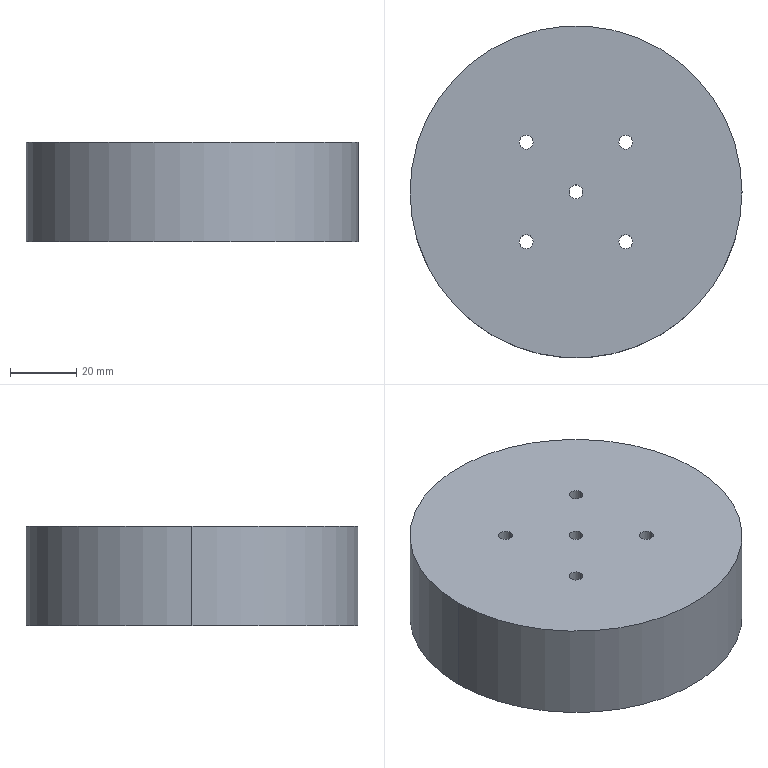Part | SolidWorks | features Extrusion 1, HoleWzd 1 | 1 solid | 14 faces | box 100 x 100 x 30 mm | volume 233541 mm3 | cylinder 12 | plane 2 | commonest cylinder face diameters 4.2 x10 100 x2
STEP:
#1=CARTESIAN_POINT('',(2.1,0.,30.));
#2=VERTEX_POINT('',#1);
#3=CARTESIAN_POINT('',(-2.1,0.,30.));
#4=VERTEX_POINT('',#3);
#5=CARTESIAN_POINT('',(0.,0.,30.));
#6=DIRECTION('',(0.,0.,-1.));
#7=DIRECTION('',(-1.,0.,0.));
#8=AXIS2_PLACEMENT_3D('',#5,#6,#7);
#9=CIRCLE('',#8,2.1);
#10=EDGE_CURVE('',#2,#4,#9,.T.);
#11=ORIENTED_EDGE('',*,*,#10,.F.);
#12=CARTESIAN_POINT('',(2.1,0.,0.));
#13=VERTEX_POINT('',#12);
#14=CARTESIAN_POINT('',(2.1,0.,0.));
#15=DIRECTION('',(0.,0.,-1.));
#16=VECTOR('',#15,1000.);
#17=LINE('',#14,#16);
#18=EDGE_CURVE('',#2,#13,#17,.T.);
#19=ORIENTED_EDGE('',*,*,#18,.T.);
#20=CARTESIAN_POINT('',(-2.1,0.,0.));
#21=VERTEX_POINT('',#20);
#22=CARTESIAN_POINT('',(0.,0.,0.));
#23=DIRECTION('',(0.,0.,-1.));
#24=DIRECTION('',(-1.,0.,0.));
#25=AXIS2_PLACEMENT_3D('',#22,#23,#24);
#26=CIRCLE('',#25,2.1);
#27=EDGE_CURVE('',#13,#21,#26,.T.);
#28=ORIENTED_EDGE('',*,*,#27,.T.);
#29=CARTESIAN_POINT('',(-2.1,0.,0.));
#30=DIRECTION('',(0.,0.,-1.));
#31=VECTOR('',#30,1000.);
#32=LINE('',#29,#31);
#33=EDGE_CURVE('',#4,#21,#32,.T.);
#34=ORIENTED_EDGE('',*,*,#33,.F.);
#35=EDGE_LOOP('',(#11,#19,#28,#34));
#36=FACE_OUTER_BOUND('',#35,.T.);
#37=CARTESIAN_POINT('',(0.,0.,0.));
#38=DIRECTION('',(0.,0.,-1.));
#39=DIRECTION('',(-1.,0.,0.));
#40=AXIS2_PLACEMENT_3D('',#37,#38,#39);
#41=CYLINDRICAL_SURFACE('',#40,2.1);
#42=ADVANCED_FACE('',(#36),#41,.F.);
#43=CARTESIAN_POINT('',(-12.9,-15.,30.));
#44=VERTEX_POINT('',#43);
#45=CARTESIAN_POINT('',(-17.1,-15.,30.));
#46=VERTEX_POINT('',#45);
#47=CARTESIAN_POINT('',(-15.,-15.,30.));
#48=DIRECTION('',(0.,0.,-1.));
#49=DIRECTION('',(-1.,0.,0.));
#50=AXIS2_PLACEMENT_3D('',#47,#48,#49);
#51=CIRCLE('',#50,2.1);
#52=EDGE_CURVE('',#44,#46,#51,.T.);
#53=ORIENTED_EDGE('',*,*,#52,.F.);
#54=CARTESIAN_POINT('',(-12.9,-15.,0.));
#55=VERTEX_POINT('',#54);
#56=CARTESIAN_POINT('',(-12.9,-15.,0.));
#57=DIRECTION('',(0.,0.,-1.));
#58=VECTOR('',#57,1000.);
#59=LINE('',#56,#58);
#60=EDGE_CURVE('',#44,#55,#59,.T.);
#61=ORIENTED_EDGE('',*,*,#60,.T.);
#62=CARTESIAN_POINT('',(-17.1,-15.,0.));
#63=VERTEX_POINT('',#62);
#64=CARTESIAN_POINT('',(-15.,-15.,0.));
#65=DIRECTION('',(0.,0.,-1.));
#66=DIRECTION('',(-1.,0.,0.));
#67=AXIS2_PLACEMENT_3D('',#64,#65,#66);
#68=CIRCLE('',#67,2.1);
#69=EDGE_CURVE('',#55,#63,#68,.T.);
#70=ORIENTED_EDGE('',*,*,#69,.T.);
#71=CARTESIAN_POINT('',(-17.1,-15.,0.));
#72=DIRECTION('',(0.,0.,-1.));
#73=VECTOR('',#72,1000.);
#74=LINE('',#71,#73);
#75=EDGE_CURVE('',#46,#63,#74,.T.);
#76=ORIENTED_EDGE('',*,*,#75,.F.);
#77=EDGE_LOOP('',(#53,#61,#70,#76));
#78=FACE_OUTER_BOUND('',#77,.T.);
#79=CARTESIAN_POINT('',(-15.,-15.,0.));
#80=DIRECTION('',(0.,0.,-1.));
#81=DIRECTION('',(-1.,0.,0.));
#82=AXIS2_PLACEMENT_3D('',#79,#80,#81);
#83=CYLINDRICAL_SURFACE('',#82,2.1);
#84=ADVANCED_FACE('',(#78),#83,.F.);
#85=CARTESIAN_POINT('',(17.1,15.,30.));
#86=VERTEX_POINT('',#85);
#87=CARTESIAN_POINT('',(12.9,15.,30.));
#88=VERTEX_POINT('',#87);
#89=CARTESIAN_POINT('',(15.,15.,30.));
#90=DIRECTION('',(0.,0.,-1.));
#91=DIRECTION('',(-1.,0.,0.));
#92=AXIS2_PLACEMENT_3D('',#89,#90,#91);
#93=CIRCLE('',#92,2.1);
#94=EDGE_CURVE('',#86,#88,#93,.T.);
#95=ORIENTED_EDGE('',*,*,#94,.F.);
#96=CARTESIAN_POINT('',(17.1,15.,0.));
#97=VERTEX_POINT('',#96);
#98=CARTESIAN_POINT('',(17.1,15.,0.));
#99=DIRECTION('',(0.,0.,-1.));
#100=VECTOR('',#99,1000.);
#101=LINE('',#98,#100);
#102=EDGE_CURVE('',#86,#97,#101,.T.);
#103=ORIENTED_EDGE('',*,*,#102,.T.);
#104=CARTESIAN_POINT('',(12.9,15.,0.));
#105=VERTEX_POINT('',#104);
#106=CARTESIAN_POINT('',(15.,15.,0.));
#107=DIRECTION('',(0.,0.,-1.));
#108=DIRECTION('',(-1.,0.,0.));
#109=AXIS2_PLACEMENT_3D('',#106,#107,#108);
#110=CIRCLE('',#109,2.1);
#111=EDGE_CURVE('',#97,#105,#110,.T.);
#112=ORIENTED_EDGE('',*,*,#111,.T.);
#113=CARTESIAN_POINT('',(12.9,15.,0.));
#114=DIRECTION('',(0.,0.,-1.));
#115=VECTOR('',#114,1000.);
#116=LINE('',#113,#115);
#117=EDGE_CURVE('',#88,#105,#116,.T.);
#118=ORIENTED_EDGE('',*,*,#117,.F.);
#119=EDGE_LOOP('',(#95,#103,#112,#118));
#120=FACE_OUTER_BOUND('',#119,.T.);
#121=CARTESIAN_POINT('',(15.,15.,0.));
#122=DIRECTION('',(0.,0.,-1.));
#123=DIRECTION('',(-1.,0.,0.));
#124=AXIS2_PLACEMENT_3D('',#121,#122,#123);
#125=CYLINDRICAL_SURFACE('',#124,2.1);
#126=ADVANCED_FACE('',(#120),#125,.F.);
#127=CARTESIAN_POINT('',(17.1,-15.,30.));
#128=VERTEX_POINT('',#127);
#129=CARTESIAN_POINT('',(12.9,-15.,30.));
#130=VERTEX_POINT('',#129);
#131=CARTESIAN_POINT('',(15.,-15.,30.));
#132=DIRECTION('',(0.,0.,-1.));
#133=DIRECTION('',(-1.,0.,0.));
#134=AXIS2_PLACEMENT_3D('',#131,#132,#133);
#135=CIRCLE('',#134,2.1);
#136=EDGE_CURVE('',#128,#130,#135,.T.);
#137=ORIENTED_EDGE('',*,*,#136,.F.);
#138=CARTESIAN_POINT('',(17.1,-15.,0.));
#139=VERTEX_POINT('',#138);
#140=CARTESIAN_POINT('',(17.1,-15.,0.));
#141=DIRECTION('',(0.,0.,-1.));
#142=VECTOR('',#141,1000.);
#143=LINE('',#140,#142);
#144=EDGE_CURVE('',#128,#139,#143,.T.);
#145=ORIENTED_EDGE('',*,*,#144,.T.);
#146=CARTESIAN_POINT('',(12.9,-15.,0.));
#147=VERTEX_POINT('',#146);
#148=CARTESIAN_POINT('',(15.,-15.,0.));
#149=DIRECTION('',(0.,0.,-1.));
#150=DIRECTION('',(-1.,0.,0.));
#151=AXIS2_PLACEMENT_3D('',#148,#149,#150);
#152=CIRCLE('',#151,2.1);
#153=EDGE_CURVE('',#139,#147,#152,.T.);
#154=ORIENTED_EDGE('',*,*,#153,.T.);
#155=CARTESIAN_POINT('',(12.9,-15.,0.));
#156=DIRECTION('',(0.,0.,-1.));
#157=VECTOR('',#156,1000.);
#158=LINE('',#155,#157);
#159=EDGE_CURVE('',#130,#147,#158,.T.);
#160=ORIENTED_EDGE('',*,*,#159,.F.);
#161=EDGE_LOOP('',(#137,#145,#154,#160));
#162=FACE_OUTER_BOUND('',#161,.T.);
#163=CARTESIAN_POINT('',(15.,-15.,0.));
#164=DIRECTION('',(0.,0.,-1.));
#165=DIRECTION('',(-1.,0.,0.));
#166=AXIS2_PLACEMENT_3D('',#163,#164,#165);
#167=CYLINDRICAL_SURFACE('',#166,2.1);
#168=ADVANCED_FACE('',(#162),#167,.F.);
#169=CARTESIAN_POINT('',(-12.9,15.,30.));
#170=VERTEX_POINT('',#169);
#171=CARTESIAN_POINT('',(-17.1,15.,30.));
#172=VERTEX_POINT('',#171);
#173=CARTESIAN_POINT('',(-15.,15.,30.));
#174=DIRECTION('',(0.,0.,-1.));
#175=DIRECTION('',(-1.,0.,0.));
#176=AXIS2_PLACEMENT_3D('',#173,#174,#175);
#177=CIRCLE('',#176,2.1);
#178=EDGE_CURVE('',#170,#172,#177,.T.);
#179=ORIENTED_EDGE('',*,*,#178,.F.);
#180=CARTESIAN_POINT('',(-12.9,15.,0.));
#181=VERTEX_POINT('',#180);
#182=CARTESIAN_POINT('',(-12.9,15.,0.));
#183=DIRECTION('',(0.,0.,-1.));
#184=VECTOR('',#183,1000.);
#185=LINE('',#182,#184);
#186=EDGE_CURVE('',#170,#181,#185,.T.);
#187=ORIENTED_EDGE('',*,*,#186,.T.);
#188=CARTESIAN_POINT('',(-17.1,15.,0.));
#189=VERTEX_POINT('',#188);
#190=CARTESIAN_POINT('',(-15.,15.,0.));
#191=DIRECTION('',(0.,0.,-1.));
#192=DIRECTION('',(-1.,0.,0.));
#193=AXIS2_PLACEMENT_3D('',#190,#191,#192);
#194=CIRCLE('',#193,2.1);
#195=EDGE_CURVE('',#181,#189,#194,.T.);
#196=ORIENTED_EDGE('',*,*,#195,.T.);
#197=CARTESIAN_POINT('',(-17.1,15.,0.));
#198=DIRECTION('',(0.,0.,-1.));
#199=VECTOR('',#198,1000.);
#200=LINE('',#197,#199);
#201=EDGE_CURVE('',#172,#189,#200,.T.);
#202=ORIENTED_EDGE('',*,*,#201,.F.);
#203=EDGE_LOOP('',(#179,#187,#196,#202));
#204=FACE_OUTER_BOUND('',#203,.T.);
#205=CARTESIAN_POINT('',(-15.,15.,0.));
#206=DIRECTION('',(0.,0.,-1.));
#207=DIRECTION('',(-1.,0.,0.));
#208=AXIS2_PLACEMENT_3D('',#205,#206,#207);
#209=CYLINDRICAL_SURFACE('',#208,2.1);
#210=ADVANCED_FACE('',(#204),#209,.F.);
#211=CARTESIAN_POINT('',(50.,0.,30.));
#212=VERTEX_POINT('',#211);
#213=CARTESIAN_POINT('',(-50.,0.,30.));
#214=VERTEX_POINT('',#213);
#215=CARTESIAN_POINT('',(0.,0.,30.));
#216=DIRECTION('',(0.,0.,1.));
#217=DIRECTION('',(1.,0.,0.));
#218=AXIS2_PLACEMENT_3D('',#215,#216,#217);
#219=CIRCLE('',#218,50.);
#220=EDGE_CURVE('',#212,#214,#219,.T.);
#221=ORIENTED_EDGE('',*,*,#220,.F.);
#222=CARTESIAN_POINT('',(50.,0.,0.));
#223=VERTEX_POINT('',#222);
#224=CARTESIAN_POINT('',(50.,0.,30.));
#225=DIRECTION('',(0.,0.,-1.));
#226=VECTOR('',#225,1000.);
#227=LINE('',#224,#226);
#228=EDGE_CURVE('',#212,#223,#227,.T.);
#229=ORIENTED_EDGE('',*,*,#228,.T.);
#230=CARTESIAN_POINT('',(-50.,0.,0.));
#231=VERTEX_POINT('',#230);
#232=CARTESIAN_POINT('',(0.,0.,0.));
#233=DIRECTION('',(0.,0.,1.));
#234=DIRECTION('',(1.,0.,0.));
#235=AXIS2_PLACEMENT_3D('',#232,#233,#234);
#236=CIRCLE('',#235,50.);
#237=EDGE_CURVE('',#223,#231,#236,.T.);
#238=ORIENTED_EDGE('',*,*,#237,.T.);
#239=CARTESIAN_POINT('',(-50.,0.,30.));
#240=DIRECTION('',(0.,0.,-1.));
#241=VECTOR('',#240,1000.);
#242=LINE('',#239,#241);
#243=EDGE_CURVE('',#214,#231,#242,.T.);
#244=ORIENTED_EDGE('',*,*,#243,.F.);
#245=EDGE_LOOP('',(#221,#229,#238,#244));
#246=FACE_OUTER_BOUND('',#245,.T.);
#247=CARTESIAN_POINT('',(0.,0.,30.));
#248=DIRECTION('',(0.,0.,-1.));
#249=DIRECTION('',(-1.,0.,0.));
#250=AXIS2_PLACEMENT_3D('',#247,#248,#249);
#251=CYLINDRICAL_SURFACE('',#250,50.);
#252=ADVANCED_FACE('',(#246),#251,.T.);
#253=ORIENTED_EDGE('',*,*,#228,.F.);
#254=CARTESIAN_POINT('',(0.,0.,30.));
#255=DIRECTION('',(0.,0.,1.));
#256=DIRECTION('',(1.,0.,0.));
#257=AXIS2_PLACEMENT_3D('',#254,#255,#256);
#258=CIRCLE('',#257,50.);
#259=EDGE_CURVE('',#214,#212,#258,.T.);
#260=ORIENTED_EDGE('',*,*,#259,.F.);
#261=ORIENTED_EDGE('',*,*,#243,.T.);
#262=CARTESIAN_POINT('',(0.,0.,0.));
#263=DIRECTION('',(0.,0.,1.));
#264=DIRECTION('',(1.,0.,0.));
#265=AXIS2_PLACEMENT_3D('',#262,#263,#264);
#266=CIRCLE('',#265,50.);
#267=EDGE_CURVE('',#231,#223,#266,.T.);
#268=ORIENTED_EDGE('',*,*,#267,.T.);
#269=EDGE_LOOP('',(#253,#260,#261,#268));
#270=FACE_OUTER_BOUND('',#269,.T.);
#271=CARTESIAN_POINT('',(0.,0.,30.));
#272=DIRECTION('',(0.,0.,-1.));
#273=DIRECTION('',(-1.,0.,0.));
#274=AXIS2_PLACEMENT_3D('',#271,#272,#273);
#275=CYLINDRICAL_SURFACE('',#274,50.);
#276=ADVANCED_FACE('',(#270),#275,.T.);
#277=CARTESIAN_POINT('',(0.,0.,30.));
#278=DIRECTION('',(0.,0.,-1.));
#279=DIRECTION('',(-1.,0.,0.));
#280=AXIS2_PLACEMENT_3D('',#277,#278,#279);
#281=CIRCLE('',#280,2.1);
#282=EDGE_CURVE('',#4,#2,#281,.T.);
#283=ORIENTED_EDGE('',*,*,#282,.T.);
#284=ORIENTED_EDGE('',*,*,#10,.T.);
#285=EDGE_LOOP('',(#283,#284));
#286=FACE_BOUND('',#285,.T.);
#287=CARTESIAN_POINT('',(-15.,-15.,30.));
#288=DIRECTION('',(0.,0.,-1.));
#289=DIRECTION('',(-1.,0.,0.));
#290=AXIS2_PLACEMENT_3D('',#287,#288,#289);
#291=CIRCLE('',#290,2.1);
#292=EDGE_CURVE('',#46,#44,#291,.T.);
#293=ORIENTED_EDGE('',*,*,#292,.T.);
#294=ORIENTED_EDGE('',*,*,#52,.T.);
#295=EDGE_LOOP('',(#293,#294));
#296=FACE_BOUND('',#295,.T.);
#297=CARTESIAN_POINT('',(15.,15.,30.));
#298=DIRECTION('',(0.,0.,-1.));
#299=DIRECTION('',(-1.,0.,0.));
#300=AXIS2_PLACEMENT_3D('',#297,#298,#299);
#301=CIRCLE('',#300,2.1);
#302=EDGE_CURVE('',#88,#86,#301,.T.);
#303=ORIENTED_EDGE('',*,*,#302,.T.);
#304=ORIENTED_EDGE('',*,*,#94,.T.);
#305=EDGE_LOOP('',(#303,#304));
#306=FACE_BOUND('',#305,.T.);
#307=CARTESIAN_POINT('',(15.,-15.,30.));
#308=DIRECTION('',(0.,0.,-1.));
#309=DIRECTION('',(-1.,0.,0.));
#310=AXIS2_PLACEMENT_3D('',#307,#308,#309);
#311=CIRCLE('',#310,2.1);
#312=EDGE_CURVE('',#130,#128,#311,.T.);
#313=ORIENTED_EDGE('',*,*,#312,.T.);
#314=ORIENTED_EDGE('',*,*,#136,.T.);
#315=EDGE_LOOP('',(#313,#314));
#316=FACE_BOUND('',#315,.T.);
#317=CARTESIAN_POINT('',(-15.,15.,30.));
#318=DIRECTION('',(0.,0.,-1.));
#319=DIRECTION('',(-1.,0.,0.));
#320=AXIS2_PLACEMENT_3D('',#317,#318,#319);
#321=CIRCLE('',#320,2.1);
#322=EDGE_CURVE('',#172,#170,#321,.T.);
#323=ORIENTED_EDGE('',*,*,#322,.T.);
#324=ORIENTED_EDGE('',*,*,#178,.T.);
#325=EDGE_LOOP('',(#323,#324));
#326=FACE_BOUND('',#325,.T.);
#327=ORIENTED_EDGE('',*,*,#259,.T.);
#328=ORIENTED_EDGE('',*,*,#220,.T.);
#329=EDGE_LOOP('',(#327,#328));
#330=FACE_OUTER_BOUND('',#329,.T.);
#331=CARTESIAN_POINT('',(0.,0.,30.));
#332=DIRECTION('',(0.,0.,1.));
#333=DIRECTION('',(1.,0.,0.));
#334=AXIS2_PLACEMENT_3D('',#331,#332,#333);
#335=PLANE('',#334);
#336=ADVANCED_FACE('',(#286,#296,#306,#316,#326,#330),#335,.T.);
#337=CARTESIAN_POINT('',(0.,0.,0.));
#338=DIRECTION('',(0.,0.,-1.));
#339=DIRECTION('',(-1.,0.,0.));
#340=AXIS2_PLACEMENT_3D('',#337,#338,#339);
#341=CIRCLE('',#340,2.1);
#342=EDGE_CURVE('',#21,#13,#341,.T.);
#343=ORIENTED_EDGE('',*,*,#342,.F.);
#344=ORIENTED_EDGE('',*,*,#27,.F.);
#345=EDGE_LOOP('',(#343,#344));
#346=FACE_BOUND('',#345,.T.);
#347=CARTESIAN_POINT('',(-15.,-15.,0.));
#348=DIRECTION('',(0.,0.,-1.));
#349=DIRECTION('',(-1.,0.,0.));
#350=AXIS2_PLACEMENT_3D('',#347,#348,#349);
#351=CIRCLE('',#350,2.1);
#352=EDGE_CURVE('',#63,#55,#351,.T.);
#353=ORIENTED_EDGE('',*,*,#352,.F.);
#354=ORIENTED_EDGE('',*,*,#69,.F.);
#355=EDGE_LOOP('',(#353,#354));
#356=FACE_BOUND('',#355,.T.);
#357=CARTESIAN_POINT('',(15.,15.,0.));
#358=DIRECTION('',(0.,0.,-1.));
#359=DIRECTION('',(-1.,0.,0.));
#360=AXIS2_PLACEMENT_3D('',#357,#358,#359);
#361=CIRCLE('',#360,2.1);
#362=EDGE_CURVE('',#105,#97,#361,.T.);
#363=ORIENTED_EDGE('',*,*,#362,.F.);
#364=ORIENTED_EDGE('',*,*,#111,.F.);
#365=EDGE_LOOP('',(#363,#364));
#366=FACE_BOUND('',#365,.T.);
#367=CARTESIAN_POINT('',(15.,-15.,0.));
#368=DIRECTION('',(0.,0.,-1.));
#369=DIRECTION('',(-1.,0.,0.));
#370=AXIS2_PLACEMENT_3D('',#367,#368,#369);
#371=CIRCLE('',#370,2.1);
#372=EDGE_CURVE('',#147,#139,#371,.T.);
#373=ORIENTED_EDGE('',*,*,#372,.F.);
#374=ORIENTED_EDGE('',*,*,#153,.F.);
#375=EDGE_LOOP('',(#373,#374));
#376=FACE_BOUND('',#375,.T.);
#377=CARTESIAN_POINT('',(-15.,15.,0.));
#378=DIRECTION('',(0.,0.,-1.));
#379=DIRECTION('',(-1.,0.,0.));
#380=AXIS2_PLACEMENT_3D('',#377,#378,#379);
#381=CIRCLE('',#380,2.1);
#382=EDGE_CURVE('',#189,#181,#381,.T.);
#383=ORIENTED_EDGE('',*,*,#382,.F.);
#384=ORIENTED_EDGE('',*,*,#195,.F.);
#385=EDGE_LOOP('',(#383,#384));
#386=FACE_BOUND('',#385,.T.);
#387=ORIENTED_EDGE('',*,*,#267,.F.);
#388=ORIENTED_EDGE('',*,*,#237,.F.);
#389=EDGE_LOOP('',(#387,#388));
#390=FACE_OUTER_BOUND('',#389,.T.);
#391=CARTESIAN_POINT('',(0.,0.,0.));
#392=DIRECTION('',(0.,0.,1.));
#393=DIRECTION('',(1.,0.,0.));
#394=AXIS2_PLACEMENT_3D('',#391,#392,#393);
#395=PLANE('',#394);
#396=ADVANCED_FACE('',(#346,#356,#366,#376,#386,#390),#395,.F.);
#397=ORIENTED_EDGE('',*,*,#186,.F.);
#398=ORIENTED_EDGE('',*,*,#322,.F.);
#399=ORIENTED_EDGE('',*,*,#201,.T.);
#400=ORIENTED_EDGE('',*,*,#382,.T.);
#401=EDGE_LOOP('',(#397,#398,#399,#400));
#402=FACE_OUTER_BOUND('',#401,.T.);
#403=CARTESIAN_POINT('',(-15.,15.,0.));
#404=DIRECTION('',(0.,0.,-1.));
#405=DIRECTION('',(-1.,0.,0.));
#406=AXIS2_PLACEMENT_3D('',#403,#404,#405);
#407=CYLINDRICAL_SURFACE('',#406,2.1);
#408=ADVANCED_FACE('',(#402),#407,.F.);
#409=ORIENTED_EDGE('',*,*,#144,.F.);
#410=ORIENTED_EDGE('',*,*,#312,.F.);
#411=ORIENTED_EDGE('',*,*,#159,.T.);
#412=ORIENTED_EDGE('',*,*,#372,.T.);
#413=EDGE_LOOP('',(#409,#410,#411,#412));
#414=FACE_OUTER_BOUND('',#413,.T.);
#415=CARTESIAN_POINT('',(15.,-15.,0.));
#416=DIRECTION('',(0.,0.,-1.));
#417=DIRECTION('',(-1.,0.,0.));
#418=AXIS2_PLACEMENT_3D('',#415,#416,#417);
#419=CYLINDRICAL_SURFACE('',#418,2.1);
#420=ADVANCED_FACE('',(#414),#419,.F.);
#421=ORIENTED_EDGE('',*,*,#102,.F.);
#422=ORIENTED_EDGE('',*,*,#302,.F.);
#423=ORIENTED_EDGE('',*,*,#117,.T.);
#424=ORIENTED_EDGE('',*,*,#362,.T.);
#425=EDGE_LOOP('',(#421,#422,#423,#424));
#426=FACE_OUTER_BOUND('',#425,.T.);
#427=CARTESIAN_POINT('',(15.,15.,0.));
#428=DIRECTION('',(0.,0.,-1.));
#429=DIRECTION('',(-1.,0.,0.));
#430=AXIS2_PLACEMENT_3D('',#427,#428,#429);
#431=CYLINDRICAL_SURFACE('',#430,2.1);
#432=ADVANCED_FACE('',(#426),#431,.F.);
#433=ORIENTED_EDGE('',*,*,#60,.F.);
#434=ORIENTED_EDGE('',*,*,#292,.F.);
#435=ORIENTED_EDGE('',*,*,#75,.T.);
#436=ORIENTED_EDGE('',*,*,#352,.T.);
#437=EDGE_LOOP('',(#433,#434,#435,#436));
#438=FACE_OUTER_BOUND('',#437,.T.);
#439=CARTESIAN_POINT('',(-15.,-15.,0.));
#440=DIRECTION('',(0.,0.,-1.));
#441=DIRECTION('',(-1.,0.,0.));
#442=AXIS2_PLACEMENT_3D('',#439,#440,#441);
#443=CYLINDRICAL_SURFACE('',#442,2.1);
#444=ADVANCED_FACE('',(#438),#443,.F.);
#445=ORIENTED_EDGE('',*,*,#18,.F.);
#446=ORIENTED_EDGE('',*,*,#282,.F.);
#447=ORIENTED_EDGE('',*,*,#33,.T.);
#448=ORIENTED_EDGE('',*,*,#342,.T.);
#449=EDGE_LOOP('',(#445,#446,#447,#448));
#450=FACE_OUTER_BOUND('',#449,.T.);
#451=CARTESIAN_POINT('',(0.,0.,0.));
#452=DIRECTION('',(0.,0.,-1.));
#453=DIRECTION('',(-1.,0.,0.));
#454=AXIS2_PLACEMENT_3D('',#451,#452,#453);
#455=CYLINDRICAL_SURFACE('',#454,2.1);
#456=ADVANCED_FACE('',(#450),#455,.F.);
#457=CLOSED_SHELL('',(#42,#84,#126,#168,#210,#252,#276,#336,#396,#408,#420,#432,#444,#456));
#458=MANIFOLD_SOLID_BREP('',#457);
#459=CARTESIAN_POINT('',(0.,0.,0.));
#460=DIRECTION('',(0.,0.,1.));
#461=DIRECTION('',(1.,0.,0.));
#462=AXIS2_PLACEMENT_3D('',#459,#460,#461);
#463=(LENGTH_UNIT()NAMED_UNIT(*)SI_UNIT(.MILLI.,.METRE.));
#464=UNCERTAINTY_MEASURE_WITH_UNIT(LENGTH_MEASURE(0.00001),#463,'','');
#465=(NAMED_UNIT(*)PLANE_ANGLE_UNIT()SI_UNIT($,.RADIAN.));
#466=(NAMED_UNIT(*)SI_UNIT($,.STERADIAN.)SOLID_ANGLE_UNIT());
#467=(GEOMETRIC_REPRESENTATION_CONTEXT(3)GLOBAL_UNCERTAINTY_ASSIGNED_CONTEXT((#464))GLOBAL_UNIT_ASSIGNED_CONTEXT((#463,#465,#466))REPRESENTATION_CONTEXT('',''));
#468=ADVANCED_BREP_SHAPE_REPRESENTATION('',(#458,#462),#467);